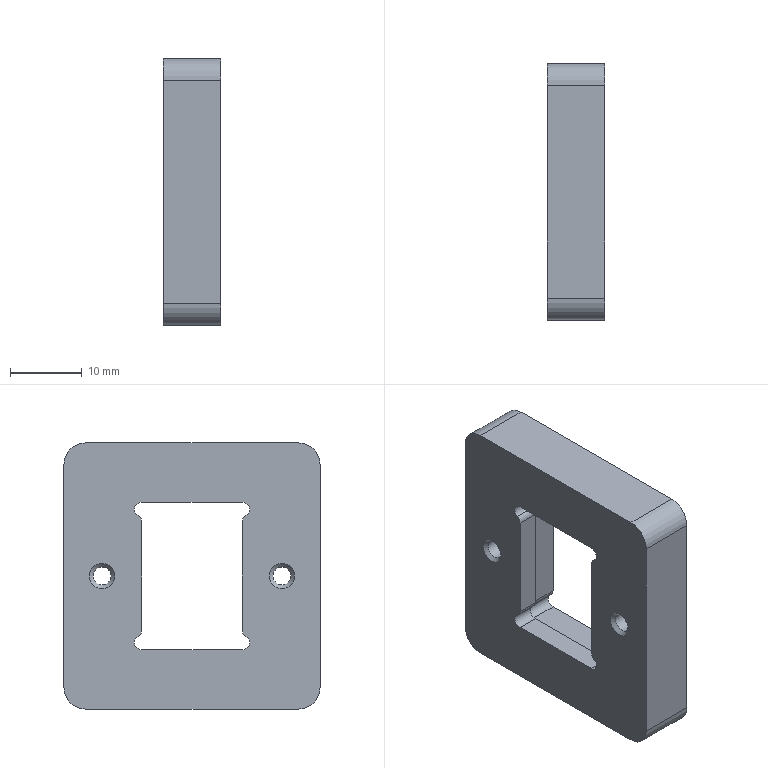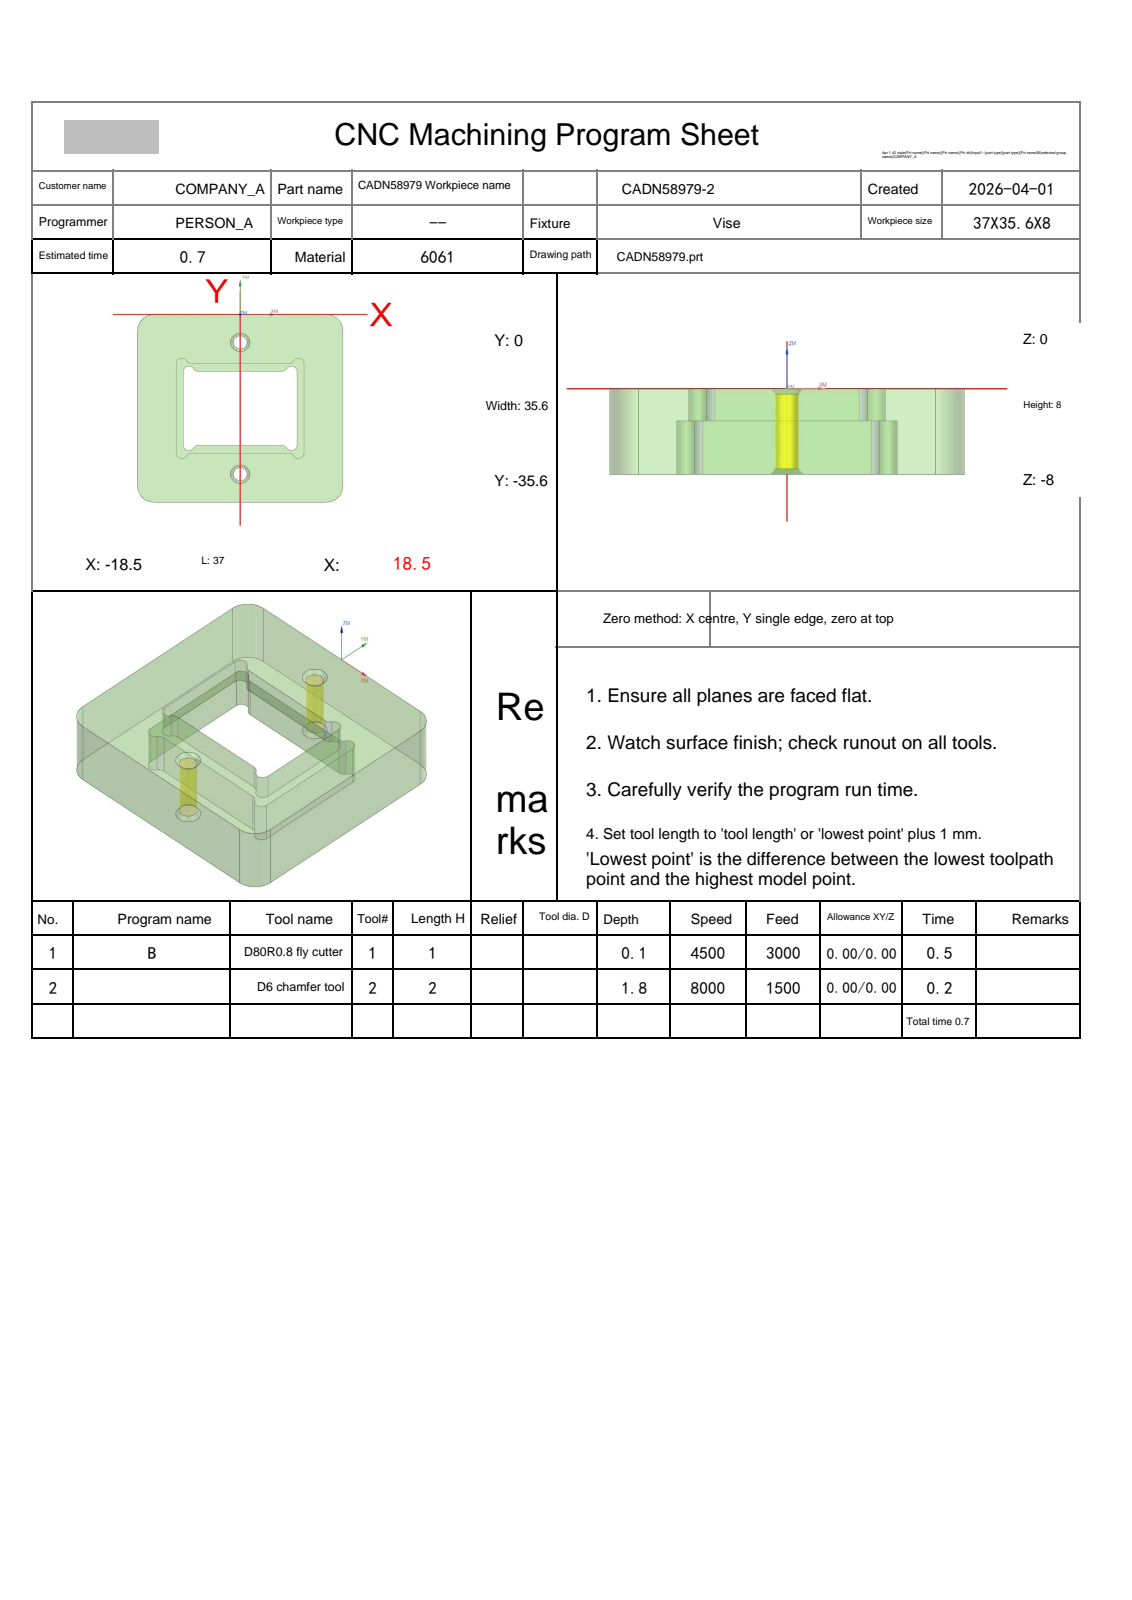NC program | NX | posted by the shop | part box 8 x 35.6 x 37 mm
Whole program:
%
O0001
(Machine time: 1.02 MIN)
(===Total Tool:2===)
(T1=D80R0.8 fly cutter D=80.  R=0.8  D-  H01 Z=-0.   )
(T2=D6 chamfer tool   D=6.   R=0.   D-  H02 Z=-1.75 )
G80 G90 G17 G49 G40
G91 G28 Z0
M01
N1 T01 M06
(D80R0.8 fly cutter  D=80. R=0.8 H=01 ce=0.20 di=0.10)
G00 G90 G54 X70.5 Y-17.8 M03 S4500
G43 H01 Z20.
M08
Z4.02
G01 Z2.02 F3000.
X58.5
X-58.5
X-70.5
Z4.02
G00 Z5.5
X70.5
Z3.54
G01 Z1.54
X58.5
X-58.5
X-70.5
Z3.54
G00 Z5.02
X70.5
Z3.06
G01 Z1.06
X58.5
X-58.5
X-70.5
Z3.06
G00 Z4.54
X70.5
Z2.58
G01 Z.58
X58.5
X-58.5
X-70.5
Z2.58
G00 Z4.06
X70.5
Z2.1
G01 Z.1
X58.5
X-58.5
X-70.5
Z2.1
G00 Z20.
G00 G90 X70.5 Y-17.8 M03 S4500
Z20.
Z2.
G01 Z0.0 F1000.
X58.5
X-58.5
X-70.5
Z2.
G00 Z20.
G91 G28 Z0.0
M05
M09
G91 G28 Z0.0
M01
N2 T02 M06
(D6 chamfer tool  D=6. R=0. H=02 ce=0.00 di=0.00)
G00 G90 G54 X0.0 Y-5.3 M03 S8000
G43 H02 Z20.
M08
G98 G81 X0.0 Y-5.3 Z-1.75 R3. F1000.
Y-30.3
G80
G00 Z20.
G00 G90 X.386 Y-36.827 M03 S6500
Z20.
Z.172
G01 Z-1.199 F1500.
G03 X.1 Y-36.627 I-1.286 J-1.532
G01 X.054 Y-36.597
X0.0 Y-36.6
X-15.5
G02 X-19.5 Y-32.6 I0.0 J4.
G01 Y-3.
G02 X-15.5 Y1. I4. J0.0
G01 X15.5
G02 X19.5 Y-3. I0.0 J-4.
G01 Y-32.6
G02 X15.5 Y-36.6 I-4. J0.0
G01 X0.0
X-.054 Y-36.597
X-.1 Y-36.627
G03 X-.386 Y-36.827 I1. J-1.732
G01 Z.172
G00 Z10.
X-9.023 Y-17.414
Z.172
G01 Z-1.199
G03 X-9.223 Y-17.7 I1.532 J-1.286
G01 X-9.253 Y-17.746
X-9.25 Y-17.8
Y-24.8
G02 X-7.518 Y-23.8 I1.732 J-1.
G01 X7.518
G02 X9.25 Y-24.8 I0.0 J-2.
G01 Y-10.8
G02 X7.518 Y-11.8 I-1.732 J1.
G01 X-7.518
G02 X-9.25 Y-10.8 I0.0 J2.
G01 Y-17.8
X-9.253 Y-17.854
X-9.223 Y-17.9
G03 X-9.023 Y-18.186 I1.732 J1.
G01 Z.172
G00 Z20.
M05
M09
G91 G28 Z0.0
G91 G28 Y0.0
M30
%